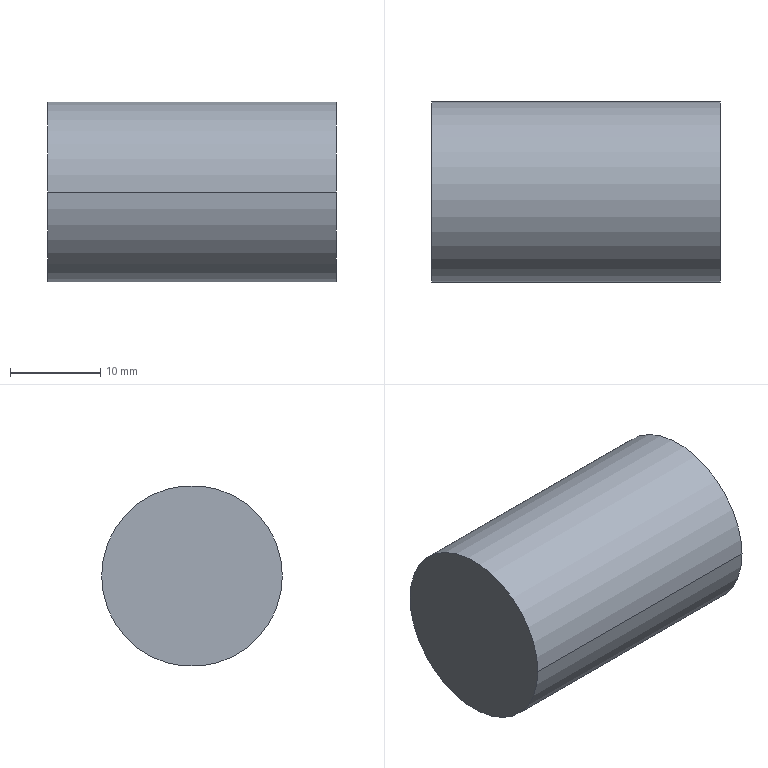Part | NX | features solid 2 | 1 solid | 4 faces | box 31.95 x 20 x 20 mm | volume 10037 mm3 | plane 2 | cylinder 2 | commonest cylinder face diameters 20 x2
STEP:
#1=CARTESIAN_POINT('',(-16.05,744.85,-1047.16));
#2=VERTEX_POINT('',#1);
#3=CARTESIAN_POINT('',(-16.05,724.85,-1047.16));
#4=VERTEX_POINT('',#3);
#5=CARTESIAN_POINT('',(-16.05,734.85,-1047.16));
#6=DIRECTION('',(1.,0.,0.));
#7=DIRECTION('',(0.,1.,0.));
#8=AXIS2_PLACEMENT_3D('',#5,#6,#7);
#9=CIRCLE('',#8,10.);
#10=EDGE_CURVE('',#2,#4,#9,.T.);
#11=ORIENTED_EDGE('',*,*,#10,.F.);
#12=CARTESIAN_POINT('',(-16.05,734.85,-1047.16));
#13=DIRECTION('',(1.,0.,0.));
#14=DIRECTION('',(0.,-1.,0.));
#15=AXIS2_PLACEMENT_3D('',#12,#13,#14);
#16=CIRCLE('',#15,10.);
#17=EDGE_CURVE('',#4,#2,#16,.T.);
#18=ORIENTED_EDGE('',*,*,#17,.F.);
#19=EDGE_LOOP('',(#11,#18));
#20=FACE_BOUND('',#19,.T.);
#21=CARTESIAN_POINT('',(-16.05,734.85,-1047.16));
#22=DIRECTION('',(1.,0.,0.));
#23=DIRECTION('',(0.,1.,0.));
#24=AXIS2_PLACEMENT_3D('',#21,#22,#23);
#25=PLANE('',#24);
#26=ADVANCED_FACE('',(#20),#25,.F.);
#27=CARTESIAN_POINT('',(15.9,744.85,-1047.16));
#28=VERTEX_POINT('',#27);
#29=CARTESIAN_POINT('',(15.9,744.85,-1047.16));
#30=DIRECTION('',(-1.,0.,0.));
#31=VECTOR('',#30,1000.);
#32=LINE('',#29,#31);
#33=EDGE_CURVE('',#28,#2,#32,.T.);
#34=ORIENTED_EDGE('',*,*,#33,.F.);
#35=CARTESIAN_POINT('',(15.9,724.85,-1047.16));
#36=VERTEX_POINT('',#35);
#37=CARTESIAN_POINT('',(15.9,734.85,-1047.16));
#38=DIRECTION('',(-1.,0.,0.));
#39=DIRECTION('',(0.,1.,0.));
#40=AXIS2_PLACEMENT_3D('',#37,#38,#39);
#41=CIRCLE('',#40,10.);
#42=EDGE_CURVE('',#28,#36,#41,.T.);
#43=ORIENTED_EDGE('',*,*,#42,.T.);
#44=CARTESIAN_POINT('',(15.9,724.85,-1047.16));
#45=DIRECTION('',(-1.,0.,0.));
#46=VECTOR('',#45,1000.);
#47=LINE('',#44,#46);
#48=EDGE_CURVE('',#4,#36,#47,.F.);
#49=ORIENTED_EDGE('',*,*,#48,.F.);
#50=ORIENTED_EDGE('',*,*,#17,.T.);
#51=EDGE_LOOP('',(#34,#43,#49,#50));
#52=FACE_BOUND('',#51,.T.);
#53=CARTESIAN_POINT('',(-16.05,734.85,-1047.16));
#54=DIRECTION('',(1.,0.,0.));
#55=DIRECTION('',(0.,1.,0.));
#56=AXIS2_PLACEMENT_3D('',#53,#54,#55);
#57=CYLINDRICAL_SURFACE('',#56,10.);
#58=ADVANCED_FACE('',(#52),#57,.T.);
#59=ORIENTED_EDGE('',*,*,#48,.T.);
#60=CARTESIAN_POINT('',(15.9,734.85,-1047.16));
#61=DIRECTION('',(-1.,0.,0.));
#62=DIRECTION('',(0.,-1.,0.));
#63=AXIS2_PLACEMENT_3D('',#60,#61,#62);
#64=CIRCLE('',#63,10.);
#65=EDGE_CURVE('',#36,#28,#64,.T.);
#66=ORIENTED_EDGE('',*,*,#65,.T.);
#67=ORIENTED_EDGE('',*,*,#33,.T.);
#68=ORIENTED_EDGE('',*,*,#10,.T.);
#69=EDGE_LOOP('',(#59,#66,#67,#68));
#70=FACE_BOUND('',#69,.T.);
#71=CARTESIAN_POINT('',(-16.05,734.85,-1047.16));
#72=DIRECTION('',(1.,0.,0.));
#73=DIRECTION('',(0.,1.,0.));
#74=AXIS2_PLACEMENT_3D('',#71,#72,#73);
#75=CYLINDRICAL_SURFACE('',#74,10.);
#76=ADVANCED_FACE('',(#70),#75,.T.);
#77=ORIENTED_EDGE('',*,*,#65,.F.);
#78=ORIENTED_EDGE('',*,*,#42,.F.);
#79=EDGE_LOOP('',(#77,#78));
#80=FACE_BOUND('',#79,.T.);
#81=CARTESIAN_POINT('',(15.9,734.85,-1047.16));
#82=DIRECTION('',(1.,0.,0.));
#83=DIRECTION('',(0.,1.,0.));
#84=AXIS2_PLACEMENT_3D('',#81,#82,#83);
#85=PLANE('',#84);
#86=ADVANCED_FACE('',(#80),#85,.T.);
#87=CLOSED_SHELL('',(#26,#58,#76,#86));
#88=MANIFOLD_SOLID_BREP('',#87);
#89=(LENGTH_UNIT()NAMED_UNIT(*)SI_UNIT(.MILLI.,.METRE.));
#90=UNCERTAINTY_MEASURE_WITH_UNIT(LENGTH_MEASURE(0.00001),#89,'','');
#91=(NAMED_UNIT(*)PLANE_ANGLE_UNIT()SI_UNIT($,.RADIAN.));
#92=(NAMED_UNIT(*)SI_UNIT($,.STERADIAN.)SOLID_ANGLE_UNIT());
#93=(GEOMETRIC_REPRESENTATION_CONTEXT(3)GLOBAL_UNCERTAINTY_ASSIGNED_CONTEXT((#90))GLOBAL_UNIT_ASSIGNED_CONTEXT((#89,#91,#92))REPRESENTATION_CONTEXT('',''));
#94=ADVANCED_BREP_SHAPE_REPRESENTATION('',(#88),#93);